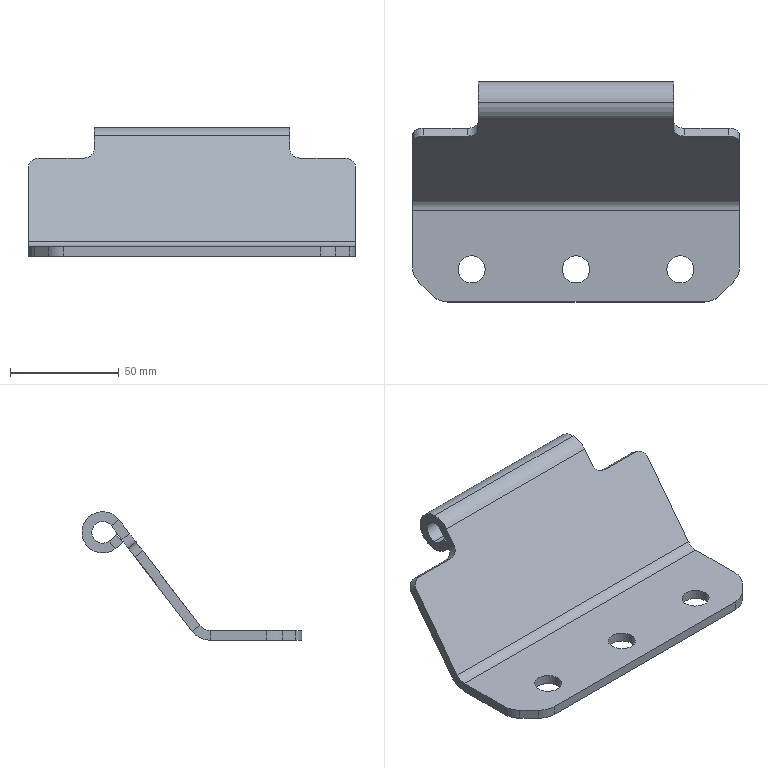Part | SolidWorks | features Fillet 2, ICE 2, Chamfer 1, FlatPattern 1, SMBaseFlange 1, SheetMetal 1 | 1 solid | 46 faces | box 150.4 x 101.2 x 59.2 mm | volume 84882 mm3 | plane 24 | cylinder 22 | commonest cylinder face diameters 10 x7 12.5 x6 20 x4 19 x3 12 x1 21 x1
STEP:
#1=CARTESIAN_POINT('',(41.75,15.,0.));
#2=VERTEX_POINT('',#1);
#3=CARTESIAN_POINT('',(54.25,15.,0.));
#4=VERTEX_POINT('',#3);
#5=CARTESIAN_POINT('',(48.,15.,0.));
#6=DIRECTION('',(0.,0.,1.));
#7=DIRECTION('',(1.,0.,0.));
#8=AXIS2_PLACEMENT_3D('',#5,#6,#7);
#9=CIRCLE('',#8,6.25);
#10=EDGE_CURVE('',#2,#4,#9,.T.);
#11=ORIENTED_EDGE('',*,*,#10,.T.);
#12=CARTESIAN_POINT('',(54.25,15.,-4.5));
#13=VERTEX_POINT('',#12);
#14=CARTESIAN_POINT('',(54.25,15.,54.7));
#15=DIRECTION('',(0.,0.,-1.));
#16=VECTOR('',#15,1000.);
#17=LINE('',#14,#16);
#18=EDGE_CURVE('',#4,#13,#17,.T.);
#19=ORIENTED_EDGE('',*,*,#18,.T.);
#20=CARTESIAN_POINT('',(41.75,15.,-4.5));
#21=VERTEX_POINT('',#20);
#22=CARTESIAN_POINT('',(48.,15.,-4.5));
#23=DIRECTION('',(0.,0.,-1.));
#24=DIRECTION('',(-1.,0.,0.));
#25=AXIS2_PLACEMENT_3D('',#22,#23,#24);
#26=CIRCLE('',#25,6.25);
#27=EDGE_CURVE('',#13,#21,#26,.T.);
#28=ORIENTED_EDGE('',*,*,#27,.T.);
#29=CARTESIAN_POINT('',(41.75,15.,54.7));
#30=DIRECTION('',(0.,0.,-1.));
#31=VECTOR('',#30,1000.);
#32=LINE('',#29,#31);
#33=EDGE_CURVE('',#2,#21,#32,.T.);
#34=ORIENTED_EDGE('',*,*,#33,.F.);
#35=EDGE_LOOP('',(#11,#19,#28,#34));
#36=FACE_OUTER_BOUND('',#35,.T.);
#37=CARTESIAN_POINT('',(48.,15.,54.7));
#38=DIRECTION('',(0.,0.,-1.));
#39=DIRECTION('',(-1.,0.,0.));
#40=AXIS2_PLACEMENT_3D('',#37,#38,#39);
#41=CYLINDRICAL_SURFACE('',#40,6.25);
#42=ADVANCED_FACE('',(#36),#41,.F.);
#43=CARTESIAN_POINT('',(-54.25,15.,0.));
#44=VERTEX_POINT('',#43);
#45=CARTESIAN_POINT('',(-41.75,15.,0.));
#46=VERTEX_POINT('',#45);
#47=CARTESIAN_POINT('',(-48.,15.,0.));
#48=DIRECTION('',(0.,0.,1.));
#49=DIRECTION('',(1.,0.,0.));
#50=AXIS2_PLACEMENT_3D('',#47,#48,#49);
#51=CIRCLE('',#50,6.25);
#52=EDGE_CURVE('',#44,#46,#51,.T.);
#53=ORIENTED_EDGE('',*,*,#52,.T.);
#54=CARTESIAN_POINT('',(-41.75,15.,-4.5));
#55=VERTEX_POINT('',#54);
#56=CARTESIAN_POINT('',(-41.75,15.,54.7));
#57=DIRECTION('',(0.,0.,-1.));
#58=VECTOR('',#57,1000.);
#59=LINE('',#56,#58);
#60=EDGE_CURVE('',#46,#55,#59,.T.);
#61=ORIENTED_EDGE('',*,*,#60,.T.);
#62=CARTESIAN_POINT('',(-54.25,15.,-4.5));
#63=VERTEX_POINT('',#62);
#64=CARTESIAN_POINT('',(-48.,15.,-4.5));
#65=DIRECTION('',(0.,0.,-1.));
#66=DIRECTION('',(-1.,0.,0.));
#67=AXIS2_PLACEMENT_3D('',#64,#65,#66);
#68=CIRCLE('',#67,6.25);
#69=EDGE_CURVE('',#55,#63,#68,.T.);
#70=ORIENTED_EDGE('',*,*,#69,.T.);
#71=CARTESIAN_POINT('',(-54.25,15.,54.7));
#72=DIRECTION('',(0.,0.,-1.));
#73=VECTOR('',#72,1000.);
#74=LINE('',#71,#73);
#75=EDGE_CURVE('',#44,#63,#74,.T.);
#76=ORIENTED_EDGE('',*,*,#75,.F.);
#77=EDGE_LOOP('',(#53,#61,#70,#76));
#78=FACE_OUTER_BOUND('',#77,.T.);
#79=CARTESIAN_POINT('',(-48.,15.,54.7));
#80=DIRECTION('',(0.,0.,-1.));
#81=DIRECTION('',(-1.,0.,0.));
#82=AXIS2_PLACEMENT_3D('',#79,#80,#81);
#83=CYLINDRICAL_SURFACE('',#82,6.25);
#84=ADVANCED_FACE('',(#78),#83,.F.);
#85=CARTESIAN_POINT('',(-6.25,15.,0.));
#86=VERTEX_POINT('',#85);
#87=CARTESIAN_POINT('',(6.25,15.,0.));
#88=VERTEX_POINT('',#87);
#89=CARTESIAN_POINT('',(0.,15.,0.));
#90=DIRECTION('',(0.,0.,1.));
#91=DIRECTION('',(1.,0.,0.));
#92=AXIS2_PLACEMENT_3D('',#89,#90,#91);
#93=CIRCLE('',#92,6.25);
#94=EDGE_CURVE('',#86,#88,#93,.T.);
#95=ORIENTED_EDGE('',*,*,#94,.T.);
#96=CARTESIAN_POINT('',(6.25,15.,-4.5));
#97=VERTEX_POINT('',#96);
#98=CARTESIAN_POINT('',(6.25,15.,54.7));
#99=DIRECTION('',(0.,0.,-1.));
#100=VECTOR('',#99,1000.);
#101=LINE('',#98,#100);
#102=EDGE_CURVE('',#88,#97,#101,.T.);
#103=ORIENTED_EDGE('',*,*,#102,.T.);
#104=CARTESIAN_POINT('',(-6.25,15.,-4.5));
#105=VERTEX_POINT('',#104);
#106=CARTESIAN_POINT('',(0.,15.,-4.5));
#107=DIRECTION('',(0.,0.,-1.));
#108=DIRECTION('',(-1.,0.,0.));
#109=AXIS2_PLACEMENT_3D('',#106,#107,#108);
#110=CIRCLE('',#109,6.25);
#111=EDGE_CURVE('',#97,#105,#110,.T.);
#112=ORIENTED_EDGE('',*,*,#111,.T.);
#113=CARTESIAN_POINT('',(-6.25,15.,54.7));
#114=DIRECTION('',(0.,0.,-1.));
#115=VECTOR('',#114,1000.);
#116=LINE('',#113,#115);
#117=EDGE_CURVE('',#86,#105,#116,.T.);
#118=ORIENTED_EDGE('',*,*,#117,.F.);
#119=EDGE_LOOP('',(#95,#103,#112,#118));
#120=FACE_OUTER_BOUND('',#119,.T.);
#121=CARTESIAN_POINT('',(0.,15.,54.7));
#122=DIRECTION('',(0.,0.,-1.));
#123=DIRECTION('',(-1.,0.,0.));
#124=AXIS2_PLACEMENT_3D('',#121,#122,#123);
#125=CYLINDRICAL_SURFACE('',#124,6.25);
#126=ADVANCED_FACE('',(#120),#125,.F.);
#127=CARTESIAN_POINT('',(45.,88.659,41.231));
#128=VERTEX_POINT('',#127);
#129=CARTESIAN_POINT('',(45.,91.7,40.2));
#130=VERTEX_POINT('',#129);
#131=CARTESIAN_POINT('',(45.,91.7,45.2));
#132=DIRECTION('',(1.,0.,0.));
#133=DIRECTION('',(0.,0.,1.));
#134=AXIS2_PLACEMENT_3D('',#131,#132,#133);
#135=CIRCLE('',#134,5.);
#136=EDGE_CURVE('',#128,#130,#135,.T.);
#137=ORIENTED_EDGE('',*,*,#136,.T.);
#138=CARTESIAN_POINT('',(-45.,91.7,40.2));
#139=VERTEX_POINT('',#138);
#140=CARTESIAN_POINT('',(75.2,91.7,40.2));
#141=DIRECTION('',(-1.,0.,0.));
#142=VECTOR('',#141,1000.);
#143=LINE('',#140,#142);
#144=EDGE_CURVE('',#130,#139,#143,.T.);
#145=ORIENTED_EDGE('',*,*,#144,.T.);
#146=CARTESIAN_POINT('',(-45.,88.659,41.231));
#147=VERTEX_POINT('',#146);
#148=CARTESIAN_POINT('',(-45.,91.7,45.2));
#149=DIRECTION('',(-1.,0.,0.));
#150=DIRECTION('',(0.,0.,-1.));
#151=AXIS2_PLACEMENT_3D('',#148,#149,#150);
#152=CIRCLE('',#151,5.);
#153=EDGE_CURVE('',#139,#147,#152,.T.);
#154=ORIENTED_EDGE('',*,*,#153,.T.);
#155=CARTESIAN_POINT('',(75.2,88.659,41.231));
#156=DIRECTION('',(-1.,0.,0.));
#157=VECTOR('',#156,1000.);
#158=LINE('',#155,#157);
#159=EDGE_CURVE('',#128,#147,#158,.T.);
#160=ORIENTED_EDGE('',*,*,#159,.F.);
#161=EDGE_LOOP('',(#137,#145,#154,#160));
#162=FACE_OUTER_BOUND('',#161,.T.);
#163=CARTESIAN_POINT('',(75.2,91.7,45.2));
#164=DIRECTION('',(-1.,0.,0.));
#165=DIRECTION('',(0.,0.,1.));
#166=AXIS2_PLACEMENT_3D('',#163,#164,#165);
#167=CYLINDRICAL_SURFACE('',#166,5.);
#168=ADVANCED_FACE('',(#162),#167,.F.);
#169=ORIENTED_EDGE('',*,*,#144,.F.);
#170=CARTESIAN_POINT('',(45.,91.7,50.2));
#171=VERTEX_POINT('',#170);
#172=CARTESIAN_POINT('',(45.,91.7,45.2));
#173=DIRECTION('',(1.,0.,0.));
#174=DIRECTION('',(0.,0.,1.));
#175=AXIS2_PLACEMENT_3D('',#172,#173,#174);
#176=CIRCLE('',#175,5.);
#177=EDGE_CURVE('',#130,#171,#176,.T.);
#178=ORIENTED_EDGE('',*,*,#177,.T.);
#179=CARTESIAN_POINT('',(-45.,91.7,50.2));
#180=VERTEX_POINT('',#179);
#181=CARTESIAN_POINT('',(75.2,91.7,50.2));
#182=DIRECTION('',(-1.,0.,0.));
#183=VECTOR('',#182,1000.);
#184=LINE('',#181,#183);
#185=EDGE_CURVE('',#171,#180,#184,.T.);
#186=ORIENTED_EDGE('',*,*,#185,.T.);
#187=CARTESIAN_POINT('',(-45.,91.7,45.2));
#188=DIRECTION('',(-1.,0.,0.));
#189=DIRECTION('',(0.,0.,-1.));
#190=AXIS2_PLACEMENT_3D('',#187,#188,#189);
#191=CIRCLE('',#190,5.);
#192=EDGE_CURVE('',#180,#139,#191,.T.);
#193=ORIENTED_EDGE('',*,*,#192,.T.);
#194=EDGE_LOOP('',(#169,#178,#186,#193));
#195=FACE_OUTER_BOUND('',#194,.T.);
#196=CARTESIAN_POINT('',(75.2,91.7,45.2));
#197=DIRECTION('',(-1.,0.,0.));
#198=DIRECTION('',(0.,0.,1.));
#199=AXIS2_PLACEMENT_3D('',#196,#197,#198);
#200=CYLINDRICAL_SURFACE('',#199,5.);
#201=ADVANCED_FACE('',(#195),#200,.F.);
#202=CARTESIAN_POINT('',(45.,91.7,35.7));
#203=VERTEX_POINT('',#202);
#204=CARTESIAN_POINT('',(45.,91.7,54.7));
#205=VERTEX_POINT('',#204);
#206=CARTESIAN_POINT('',(45.,91.7,45.2));
#207=DIRECTION('',(1.,0.,0.));
#208=DIRECTION('',(0.,0.,1.));
#209=AXIS2_PLACEMENT_3D('',#206,#207,#208);
#210=CIRCLE('',#209,9.5);
#211=EDGE_CURVE('',#203,#205,#210,.T.);
#212=ORIENTED_EDGE('',*,*,#211,.F.);
#213=CARTESIAN_POINT('',(-45.,91.7,35.7));
#214=VERTEX_POINT('',#213);
#215=CARTESIAN_POINT('',(75.2,91.7,35.7));
#216=DIRECTION('',(-1.,0.,0.));
#217=VECTOR('',#216,1000.);
#218=LINE('',#215,#217);
#219=EDGE_CURVE('',#203,#214,#218,.T.);
#220=ORIENTED_EDGE('',*,*,#219,.T.);
#221=CARTESIAN_POINT('',(-45.,91.7,54.7));
#222=VERTEX_POINT('',#221);
#223=CARTESIAN_POINT('',(-45.,91.7,45.2));
#224=DIRECTION('',(-1.,0.,0.));
#225=DIRECTION('',(0.,0.,-1.));
#226=AXIS2_PLACEMENT_3D('',#223,#224,#225);
#227=CIRCLE('',#226,9.5);
#228=EDGE_CURVE('',#222,#214,#227,.T.);
#229=ORIENTED_EDGE('',*,*,#228,.F.);
#230=CARTESIAN_POINT('',(75.2,91.7,54.7));
#231=DIRECTION('',(-1.,0.,0.));
#232=VECTOR('',#231,1000.);
#233=LINE('',#230,#232);
#234=EDGE_CURVE('',#205,#222,#233,.T.);
#235=ORIENTED_EDGE('',*,*,#234,.F.);
#236=EDGE_LOOP('',(#212,#220,#229,#235));
#237=FACE_OUTER_BOUND('',#236,.T.);
#238=CARTESIAN_POINT('',(75.2,91.7,45.2));
#239=DIRECTION('',(-1.,0.,0.));
#240=DIRECTION('',(0.,0.,1.));
#241=AXIS2_PLACEMENT_3D('',#238,#239,#240);
#242=CYLINDRICAL_SURFACE('',#241,9.5);
#243=ADVANCED_FACE('',(#237),#242,.T.);
#244=CARTESIAN_POINT('',(45.,84.159,50.978));
#245=VERTEX_POINT('',#244);
#246=CARTESIAN_POINT('',(45.,91.7,45.2));
#247=DIRECTION('',(1.,0.,0.));
#248=DIRECTION('',(0.,0.,1.));
#249=AXIS2_PLACEMENT_3D('',#246,#247,#248);
#250=CIRCLE('',#249,9.5);
#251=EDGE_CURVE('',#205,#245,#250,.T.);
#252=ORIENTED_EDGE('',*,*,#251,.F.);
#253=ORIENTED_EDGE('',*,*,#234,.T.);
#254=CARTESIAN_POINT('',(-45.,84.159,50.978));
#255=VERTEX_POINT('',#254);
#256=CARTESIAN_POINT('',(-45.,91.7,45.2));
#257=DIRECTION('',(-1.,0.,0.));
#258=DIRECTION('',(0.,0.,-1.));
#259=AXIS2_PLACEMENT_3D('',#256,#257,#258);
#260=CIRCLE('',#259,9.5);
#261=EDGE_CURVE('',#255,#222,#260,.T.);
#262=ORIENTED_EDGE('',*,*,#261,.F.);
#263=CARTESIAN_POINT('',(75.2,84.159,50.978));
#264=DIRECTION('',(-1.,0.,0.));
#265=VECTOR('',#264,1000.);
#266=LINE('',#263,#265);
#267=EDGE_CURVE('',#245,#255,#266,.T.);
#268=ORIENTED_EDGE('',*,*,#267,.F.);
#269=EDGE_LOOP('',(#252,#253,#262,#268));
#270=FACE_OUTER_BOUND('',#269,.T.);
#271=CARTESIAN_POINT('',(75.2,91.7,45.2));
#272=DIRECTION('',(-1.,0.,0.));
#273=DIRECTION('',(0.,0.,1.));
#274=AXIS2_PLACEMENT_3D('',#271,#272,#273);
#275=CYLINDRICAL_SURFACE('',#274,9.5);
#276=ADVANCED_FACE('',(#270),#275,.T.);
#277=CARTESIAN_POINT('',(-45.,85.087,43.968));
#278=VERTEX_POINT('',#277);
#279=CARTESIAN_POINT('',(-45.,88.659,41.231));
#280=DIRECTION('',(0.,-0.7938,0.6082));
#281=VECTOR('',#280,1000.);
#282=LINE('',#279,#281);
#283=EDGE_CURVE('',#147,#278,#282,.T.);
#284=ORIENTED_EDGE('',*,*,#283,.F.);
#285=CARTESIAN_POINT('',(-45.,85.922,37.659));
#286=VERTEX_POINT('',#285);
#287=CARTESIAN_POINT('',(-45.,88.659,41.231));
#288=DIRECTION('',(0.,-0.6082,-0.7938));
#289=VECTOR('',#288,1000.);
#290=LINE('',#287,#289);
#291=EDGE_CURVE('',#147,#286,#290,.T.);
#292=ORIENTED_EDGE('',*,*,#291,.T.);
#293=CARTESIAN_POINT('',(-45.,82.35,40.396));
#294=VERTEX_POINT('',#293);
#295=CARTESIAN_POINT('',(-45.,85.922,37.659));
#296=DIRECTION('',(0.,-0.7938,0.6082));
#297=VECTOR('',#296,1000.);
#298=LINE('',#295,#297);
#299=EDGE_CURVE('',#286,#294,#298,.T.);
#300=ORIENTED_EDGE('',*,*,#299,.T.);
#301=CARTESIAN_POINT('',(-45.,82.35,40.396));
#302=DIRECTION('',(0.,0.6082,0.7938));
#303=VECTOR('',#302,1000.);
#304=LINE('',#301,#303);
#305=EDGE_CURVE('',#294,#278,#304,.T.);
#306=ORIENTED_EDGE('',*,*,#305,.T.);
#307=EDGE_LOOP('',(#284,#292,#300,#306));
#308=FACE_OUTER_BOUND('',#307,.T.);
#309=CARTESIAN_POINT('',(-45.,127.458,29.77));
#310=DIRECTION('',(1.,0.,0.));
#311=DIRECTION('',(0.,0.,-1.));
#312=AXIS2_PLACEMENT_3D('',#309,#310,#311);
#313=PLANE('',#312);
#314=ADVANCED_FACE('',(#308),#313,.F.);
#315=CARTESIAN_POINT('',(-45.,82.865,41.891));
#316=VERTEX_POINT('',#315);
#317=CARTESIAN_POINT('',(-45.,87.731,48.241));
#318=VERTEX_POINT('',#317);
#319=CARTESIAN_POINT('',(-45.,48.672,-2.737));
#320=DIRECTION('',(0.,0.6082,0.7938));
#321=VECTOR('',#320,1000.);
#322=LINE('',#319,#321);
#323=EDGE_CURVE('',#316,#318,#322,.T.);
#324=ORIENTED_EDGE('',*,*,#323,.F.);
#325=CARTESIAN_POINT('',(-45.,79.293,44.628));
#326=VERTEX_POINT('',#325);
#327=CARTESIAN_POINT('',(-45.,79.293,44.628));
#328=DIRECTION('',(0.,-0.7938,0.6082));
#329=VECTOR('',#328,1000.);
#330=LINE('',#327,#329);
#331=EDGE_CURVE('',#316,#326,#330,.T.);
#332=ORIENTED_EDGE('',*,*,#331,.T.);
#333=CARTESIAN_POINT('',(-45.,89.937,58.519));
#334=DIRECTION('',(0.,0.6082,0.7938));
#335=VECTOR('',#334,1000.);
#336=LINE('',#333,#335);
#337=EDGE_CURVE('',#326,#255,#336,.T.);
#338=ORIENTED_EDGE('',*,*,#337,.T.);
#339=CARTESIAN_POINT('',(-45.,84.159,50.978));
#340=DIRECTION('',(0.,0.7938,-0.6082));
#341=VECTOR('',#340,1000.);
#342=LINE('',#339,#341);
#343=EDGE_CURVE('',#255,#318,#342,.T.);
#344=ORIENTED_EDGE('',*,*,#343,.T.);
#345=EDGE_LOOP('',(#324,#332,#338,#344));
#346=FACE_OUTER_BOUND('',#345,.T.);
#347=CARTESIAN_POINT('',(-45.,127.458,29.77));
#348=DIRECTION('',(1.,0.,0.));
#349=DIRECTION('',(0.,0.,-1.));
#350=AXIS2_PLACEMENT_3D('',#347,#348,#349);
#351=PLANE('',#350);
#352=ADVANCED_FACE('',(#346),#351,.F.);
#353=CARTESIAN_POINT('',(45.,82.35,40.396));
#354=VERTEX_POINT('',#353);
#355=CARTESIAN_POINT('',(45.,85.922,37.659));
#356=VERTEX_POINT('',#355);
#357=CARTESIAN_POINT('',(45.,85.922,37.659));
#358=DIRECTION('',(0.,0.7938,-0.6082));
#359=VECTOR('',#358,1000.);
#360=LINE('',#357,#359);
#361=EDGE_CURVE('',#354,#356,#360,.T.);
#362=ORIENTED_EDGE('',*,*,#361,.T.);
#363=CARTESIAN_POINT('',(45.,85.922,37.659));
#364=DIRECTION('',(0.,0.6082,0.7938));
#365=VECTOR('',#364,1000.);
#366=LINE('',#363,#365);
#367=EDGE_CURVE('',#356,#128,#366,.T.);
#368=ORIENTED_EDGE('',*,*,#367,.T.);
#369=CARTESIAN_POINT('',(45.,85.087,43.968));
#370=VERTEX_POINT('',#369);
#371=CARTESIAN_POINT('',(45.,88.659,41.231));
#372=DIRECTION('',(0.,0.7938,-0.6082));
#373=VECTOR('',#372,1000.);
#374=LINE('',#371,#373);
#375=EDGE_CURVE('',#370,#128,#374,.T.);
#376=ORIENTED_EDGE('',*,*,#375,.F.);
#377=CARTESIAN_POINT('',(45.,82.35,40.396));
#378=DIRECTION('',(0.,-0.6082,-0.7938));
#379=VECTOR('',#378,1000.);
#380=LINE('',#377,#379);
#381=EDGE_CURVE('',#370,#354,#380,.T.);
#382=ORIENTED_EDGE('',*,*,#381,.T.);
#383=EDGE_LOOP('',(#362,#368,#376,#382));
#384=FACE_OUTER_BOUND('',#383,.T.);
#385=CARTESIAN_POINT('',(45.,127.458,29.77));
#386=DIRECTION('',(-1.,0.,0.));
#387=DIRECTION('',(0.,0.,1.));
#388=AXIS2_PLACEMENT_3D('',#385,#386,#387);
#389=PLANE('',#388);
#390=ADVANCED_FACE('',(#384),#389,.F.);
#391=CARTESIAN_POINT('',(45.,79.293,44.628));
#392=VERTEX_POINT('',#391);
#393=CARTESIAN_POINT('',(45.,89.937,58.519));
#394=DIRECTION('',(0.,-0.6082,-0.7938));
#395=VECTOR('',#394,1000.);
#396=LINE('',#393,#395);
#397=EDGE_CURVE('',#245,#392,#396,.T.);
#398=ORIENTED_EDGE('',*,*,#397,.T.);
#399=CARTESIAN_POINT('',(45.,82.865,41.891));
#400=VERTEX_POINT('',#399);
#401=CARTESIAN_POINT('',(45.,82.865,41.891));
#402=DIRECTION('',(0.,0.7938,-0.6082));
#403=VECTOR('',#402,1000.);
#404=LINE('',#401,#403);
#405=EDGE_CURVE('',#392,#400,#404,.T.);
#406=ORIENTED_EDGE('',*,*,#405,.T.);
#407=CARTESIAN_POINT('',(45.,87.731,48.241));
#408=VERTEX_POINT('',#407);
#409=CARTESIAN_POINT('',(45.,48.672,-2.737));
#410=DIRECTION('',(0.,-0.6082,-0.7938));
#411=VECTOR('',#410,1000.);
#412=LINE('',#409,#411);
#413=EDGE_CURVE('',#408,#400,#412,.T.);
#414=ORIENTED_EDGE('',*,*,#413,.F.);
#415=CARTESIAN_POINT('',(45.,87.731,48.241));
#416=DIRECTION('',(0.,-0.7938,0.6082));
#417=VECTOR('',#416,1000.);
#418=LINE('',#415,#417);
#419=EDGE_CURVE('',#408,#245,#418,.T.);
#420=ORIENTED_EDGE('',*,*,#419,.T.);
#421=EDGE_LOOP('',(#398,#406,#414,#420));
#422=FACE_OUTER_BOUND('',#421,.T.);
#423=CARTESIAN_POINT('',(45.,127.458,29.77));
#424=DIRECTION('',(-1.,0.,0.));
#425=DIRECTION('',(0.,0.,1.));
#426=AXIS2_PLACEMENT_3D('',#423,#424,#425);
#427=PLANE('',#426);
#428=ADVANCED_FACE('',(#422),#427,.F.);
#429=CARTESIAN_POINT('',(-75.2,46.901,2.351));
#430=VERTEX_POINT('',#429);
#431=CARTESIAN_POINT('',(-75.2,73.211,36.69));
#432=VERTEX_POINT('',#431);
#433=CARTESIAN_POINT('',(-75.2,45.1,0.));
#434=DIRECTION('',(0.,0.6082,0.7938));
#435=VECTOR('',#434,1000.);
#436=LINE('',#433,#435);
#437=EDGE_CURVE('',#430,#432,#436,.T.);
#438=ORIENTED_EDGE('',*,*,#437,.T.);
#439=CARTESIAN_POINT('',(-75.2,76.784,33.953));
#440=VERTEX_POINT('',#439);
#441=CARTESIAN_POINT('',(-75.2,76.784,33.953));
#442=DIRECTION('',(0.,0.7938,-0.6082));
#443=VECTOR('',#442,1000.);
#444=LINE('',#441,#443);
#445=EDGE_CURVE('',#432,#440,#444,.T.);
#446=ORIENTED_EDGE('',*,*,#445,.T.);
#447=CARTESIAN_POINT('',(-75.2,50.473,-0.3861));
#448=VERTEX_POINT('',#447);
#449=CARTESIAN_POINT('',(-75.2,48.672,-2.737));
#450=DIRECTION('',(0.,0.6082,0.7938));
#451=VECTOR('',#450,1000.);
#452=LINE('',#449,#451);
#453=EDGE_CURVE('',#448,#440,#452,.T.);
#454=ORIENTED_EDGE('',*,*,#453,.F.);
#455=CARTESIAN_POINT('',(-75.2,50.473,-0.3861));
#456=DIRECTION('',(0.,-0.7938,0.6082));
#457=VECTOR('',#456,1000.);
#458=LINE('',#455,#457);
#459=EDGE_CURVE('',#448,#430,#458,.T.);
#460=ORIENTED_EDGE('',*,*,#459,.T.);
#461=EDGE_LOOP('',(#438,#446,#454,#460));
#462=FACE_OUTER_BOUND('',#461,.T.);
#463=CARTESIAN_POINT('',(-75.2,88.659,41.231));
#464=DIRECTION('',(-1.,0.,0.));
#465=DIRECTION('',(0.,0.,1.));
#466=AXIS2_PLACEMENT_3D('',#463,#464,#465);
#467=PLANE('',#466);
#468=ADVANCED_FACE('',(#462),#467,.T.);
#469=CARTESIAN_POINT('',(75.2,46.901,2.351));
#470=VERTEX_POINT('',#469);
#471=CARTESIAN_POINT('',(75.2,50.473,-0.3861));
#472=VERTEX_POINT('',#471);
#473=CARTESIAN_POINT('',(75.2,46.901,2.351));
#474=DIRECTION('',(0.,0.7938,-0.6082));
#475=VECTOR('',#474,1000.);
#476=LINE('',#473,#475);
#477=EDGE_CURVE('',#470,#472,#476,.T.);
#478=ORIENTED_EDGE('',*,*,#477,.F.);
#479=CARTESIAN_POINT('',(75.2,42.138,0.));
#480=VERTEX_POINT('',#479);
#481=CARTESIAN_POINT('',(75.2,42.138,6.));
#482=DIRECTION('',(1.,0.,0.));
#483=DIRECTION('',(0.,0.,1.));
#484=AXIS2_PLACEMENT_3D('',#481,#482,#483);
#485=CIRCLE('',#484,6.);
#486=EDGE_CURVE('',#480,#470,#485,.T.);
#487=ORIENTED_EDGE('',*,*,#486,.F.);
#488=CARTESIAN_POINT('',(75.2,42.138,-4.5));
#489=VERTEX_POINT('',#488);
#490=CARTESIAN_POINT('',(75.2,42.138,-4.5));
#491=DIRECTION('',(0.,0.,1.));
#492=VECTOR('',#491,1000.);
#493=LINE('',#490,#492);
#494=EDGE_CURVE('',#489,#480,#493,.T.);
#495=ORIENTED_EDGE('',*,*,#494,.F.);
#496=CARTESIAN_POINT('',(75.2,42.138,6.));
#497=DIRECTION('',(1.,0.,0.));
#498=DIRECTION('',(0.,0.,-1.));
#499=AXIS2_PLACEMENT_3D('',#496,#497,#498);
#500=CIRCLE('',#499,10.5);
#501=EDGE_CURVE('',#489,#472,#500,.T.);
#502=ORIENTED_EDGE('',*,*,#501,.T.);
#503=EDGE_LOOP('',(#478,#487,#495,#502));
#504=FACE_OUTER_BOUND('',#503,.T.);
#505=CARTESIAN_POINT('',(75.2,46.901,2.351));
#506=DIRECTION('',(1.,0.,0.));
#507=DIRECTION('',(0.,0.,-1.));
#508=AXIS2_PLACEMENT_3D('',#505,#506,#507);
#509=PLANE('',#508);
#510=ADVANCED_FACE('',(#504),#509,.T.);
#511=CARTESIAN_POINT('',(75.2,76.784,33.953));
#512=VERTEX_POINT('',#511);
#513=CARTESIAN_POINT('',(75.2,48.672,-2.737));
#514=DIRECTION('',(0.,0.6082,0.7938));
#515=VECTOR('',#514,1000.);
#516=LINE('',#513,#515);
#517=EDGE_CURVE('',#472,#512,#516,.T.);
#518=ORIENTED_EDGE('',*,*,#517,.T.);
#519=CARTESIAN_POINT('',(75.2,73.211,36.69));
#520=VERTEX_POINT('',#519);
#521=CARTESIAN_POINT('',(75.2,73.211,36.69));
#522=DIRECTION('',(0.,-0.7938,0.6082));
#523=VECTOR('',#522,1000.);
#524=LINE('',#521,#523);
#525=EDGE_CURVE('',#512,#520,#524,.T.);
#526=ORIENTED_EDGE('',*,*,#525,.T.);
#527=CARTESIAN_POINT('',(75.2,45.1,0.));
#528=DIRECTION('',(0.,0.6082,0.7938));
#529=VECTOR('',#528,1000.);
#530=LINE('',#527,#529);
#531=EDGE_CURVE('',#470,#520,#530,.T.);
#532=ORIENTED_EDGE('',*,*,#531,.F.);
#533=ORIENTED_EDGE('',*,*,#477,.T.);
#534=EDGE_LOOP('',(#518,#526,#532,#533));
#535=FACE_OUTER_BOUND('',#534,.T.);
#536=CARTESIAN_POINT('',(75.2,42.138,-4.5));
#537=DIRECTION('',(1.,0.,0.));
#538=DIRECTION('',(0.,0.,-1.));
#539=AXIS2_PLACEMENT_3D('',#536,#537,#538);
#540=PLANE('',#539);
#541=ADVANCED_FACE('',(#535),#540,.T.);
#542=CARTESIAN_POINT('',(-75.2,42.138,0.));
#543=VERTEX_POINT('',#542);
#544=CARTESIAN_POINT('',(-75.2,42.138,-4.5));
#545=VERTEX_POINT('',#544);
#546=CARTESIAN_POINT('',(-75.2,42.138,0.));
#547=DIRECTION('',(0.,0.,-1.));
#548=VECTOR('',#547,1000.);
#549=LINE('',#546,#548);
#550=EDGE_CURVE('',#543,#545,#549,.T.);
#551=ORIENTED_EDGE('',*,*,#550,.F.);
#552=CARTESIAN_POINT('',(-75.2,42.138,6.));
#553=DIRECTION('',(1.,0.,0.));
#554=DIRECTION('',(0.,0.,1.));
#555=AXIS2_PLACEMENT_3D('',#552,#553,#554);
#556=CIRCLE('',#555,6.);
#557=EDGE_CURVE('',#543,#430,#556,.T.);
#558=ORIENTED_EDGE('',*,*,#557,.T.);
#559=ORIENTED_EDGE('',*,*,#459,.F.);
#560=CARTESIAN_POINT('',(-75.2,42.138,6.));
#561=DIRECTION('',(1.,0.,0.));
#562=DIRECTION('',(0.,0.,-1.));
#563=AXIS2_PLACEMENT_3D('',#560,#561,#562);
#564=CIRCLE('',#563,10.5);
#565=EDGE_CURVE('',#545,#448,#564,.T.);
#566=ORIENTED_EDGE('',*,*,#565,.F.);
#567=EDGE_LOOP('',(#551,#558,#559,#566));
#568=FACE_OUTER_BOUND('',#567,.T.);
#569=CARTESIAN_POINT('',(-75.2,42.138,0.));
#570=DIRECTION('',(-1.,0.,0.));
#571=DIRECTION('',(0.,0.,1.));
#572=AXIS2_PLACEMENT_3D('',#569,#570,#571);
#573=PLANE('',#572);
#574=ADVANCED_FACE('',(#568),#573,.T.);
#575=CARTESIAN_POINT('',(-75.2,16.142,-4.5));
#576=VERTEX_POINT('',#575);
#577=CARTESIAN_POINT('',(-75.2,0.,-4.5));
#578=DIRECTION('',(0.,1.,0.));
#579=VECTOR('',#578,1000.);
#580=LINE('',#577,#579);
#581=EDGE_CURVE('',#576,#545,#580,.T.);
#582=ORIENTED_EDGE('',*,*,#581,.F.);
#583=CARTESIAN_POINT('',(-75.2,16.142,0.));
#584=VERTEX_POINT('',#583);
#585=CARTESIAN_POINT('',(-75.2,16.142,-0.3861));
#586=DIRECTION('',(0.,0.,1.));
#587=VECTOR('',#586,1000.);
#588=LINE('',#585,#587);
#589=EDGE_CURVE('',#576,#584,#588,.T.);
#590=ORIENTED_EDGE('',*,*,#589,.T.);
#591=CARTESIAN_POINT('',(-75.2,0.,0.));
#592=DIRECTION('',(0.,1.,0.));
#593=VECTOR('',#592,1000.);
#594=LINE('',#591,#593);
#595=EDGE_CURVE('',#584,#543,#594,.T.);
#596=ORIENTED_EDGE('',*,*,#595,.T.);
#597=ORIENTED_EDGE('',*,*,#550,.T.);
#598=EDGE_LOOP('',(#582,#590,#596,#597));
#599=FACE_OUTER_BOUND('',#598,.T.);
#600=CARTESIAN_POINT('',(-75.2,50.473,-0.3861));
#601=DIRECTION('',(-1.,0.,0.));
#602=DIRECTION('',(0.,0.,1.));
#603=AXIS2_PLACEMENT_3D('',#600,#601,#602);
#604=PLANE('',#603);
#605=ADVANCED_FACE('',(#599),#604,.T.);
#606=ORIENTED_EDGE('',*,*,#159,.T.);
#607=ORIENTED_EDGE('',*,*,#283,.T.);
#608=CARTESIAN_POINT('',(75.2,85.087,43.968));
#609=DIRECTION('',(-1.,0.,0.));
#610=VECTOR('',#609,1000.);
#611=LINE('',#608,#610);
#612=EDGE_CURVE('',#370,#278,#611,.T.);
#613=ORIENTED_EDGE('',*,*,#612,.F.);
#614=ORIENTED_EDGE('',*,*,#375,.T.);
#615=EDGE_LOOP('',(#606,#607,#613,#614));
#616=FACE_OUTER_BOUND('',#615,.T.);
#617=CARTESIAN_POINT('',(75.2,88.659,41.231));
#618=DIRECTION('',(0.,-0.6082,-0.7938));
#619=DIRECTION('',(0.,0.7938,-0.6082));
#620=AXIS2_PLACEMENT_3D('',#617,#618,#619);
#621=PLANE('',#620);
#622=ADVANCED_FACE('',(#616),#621,.F.);
#623=ORIENTED_EDGE('',*,*,#305,.F.);
#624=CARTESIAN_POINT('',(75.2,82.35,40.396));
#625=DIRECTION('',(-1.,0.,0.));
#626=VECTOR('',#625,1000.);
#627=LINE('',#624,#626);
#628=EDGE_CURVE('',#354,#294,#627,.T.);
#629=ORIENTED_EDGE('',*,*,#628,.F.);
#630=ORIENTED_EDGE('',*,*,#381,.F.);
#631=ORIENTED_EDGE('',*,*,#612,.T.);
#632=EDGE_LOOP('',(#623,#629,#630,#631));
#633=FACE_OUTER_BOUND('',#632,.T.);
#634=CARTESIAN_POINT('',(75.2,82.35,40.396));
#635=DIRECTION('',(0.,-0.7938,0.6082));
#636=DIRECTION('',(0.,-0.6082,-0.7938));
#637=AXIS2_PLACEMENT_3D('',#634,#635,#636);
#638=PLANE('',#637);
#639=ADVANCED_FACE('',(#633),#638,.T.);
#640=ORIENTED_EDGE('',*,*,#299,.F.);
#641=CARTESIAN_POINT('',(75.2,85.922,37.659));
#642=DIRECTION('',(-1.,0.,0.));
#643=VECTOR('',#642,1000.);
#644=LINE('',#641,#643);
#645=EDGE_CURVE('',#356,#286,#644,.T.);
#646=ORIENTED_EDGE('',*,*,#645,.F.);
#647=ORIENTED_EDGE('',*,*,#361,.F.);
#648=ORIENTED_EDGE('',*,*,#628,.T.);
#649=EDGE_LOOP('',(#640,#646,#647,#648));
#650=FACE_OUTER_BOUND('',#649,.T.);
#651=CARTESIAN_POINT('',(75.2,85.922,37.659));
#652=DIRECTION('',(0.,-0.6082,-0.7938));
#653=DIRECTION('',(0.,0.7938,-0.6082));
#654=AXIS2_PLACEMENT_3D('',#651,#652,#653);
#655=PLANE('',#654);
#656=ADVANCED_FACE('',(#650),#655,.T.);
#657=ORIENTED_EDGE('',*,*,#219,.F.);
#658=CARTESIAN_POINT('',(45.,91.7,45.2));
#659=DIRECTION('',(1.,0.,0.));
#660=DIRECTION('',(0.,0.,1.));
#661=AXIS2_PLACEMENT_3D('',#658,#659,#660);
#662=CIRCLE('',#661,9.5);
#663=EDGE_CURVE('',#356,#203,#662,.T.);
#664=ORIENTED_EDGE('',*,*,#663,.F.);
#665=ORIENTED_EDGE('',*,*,#645,.T.);
#666=CARTESIAN_POINT('',(-45.,91.7,45.2));
#667=DIRECTION('',(-1.,0.,0.));
#668=DIRECTION('',(0.,0.,-1.));
#669=AXIS2_PLACEMENT_3D('',#666,#667,#668);
#670=CIRCLE('',#669,9.5);
#671=EDGE_CURVE('',#214,#286,#670,.T.);
#672=ORIENTED_EDGE('',*,*,#671,.F.);
#673=EDGE_LOOP('',(#657,#664,#665,#672));
#674=FACE_OUTER_BOUND('',#673,.T.);
#675=CARTESIAN_POINT('',(75.2,91.7,45.2));
#676=DIRECTION('',(-1.,0.,0.));
#677=DIRECTION('',(0.,0.,1.));
#678=AXIS2_PLACEMENT_3D('',#675,#676,#677);
#679=CYLINDRICAL_SURFACE('',#678,9.5);
#680=ADVANCED_FACE('',(#674),#679,.T.);
#681=ORIENTED_EDGE('',*,*,#531,.T.);
#682=CARTESIAN_POINT('',(70.2,76.252,40.659));
#683=VERTEX_POINT('',#682);
#684=CARTESIAN_POINT('',(70.2,73.211,36.69));
#685=DIRECTION('',(0.,-0.7938,0.6082));
#686=DIRECTION('',(0.,-0.6082,-0.7938));
#687=AXIS2_PLACEMENT_3D('',#684,#685,#686);
#688=CIRCLE('',#687,5.);
#689=EDGE_CURVE('',#520,#683,#688,.T.);
#690=ORIENTED_EDGE('',*,*,#689,.T.);
#691=CARTESIAN_POINT('',(50.,76.252,40.659));
#692=VERTEX_POINT('',#691);
#693=CARTESIAN_POINT('',(75.2,76.252,40.659));
#694=DIRECTION('',(1.,0.,0.));
#695=VECTOR('',#694,1000.);
#696=LINE('',#693,#695);
#697=EDGE_CURVE('',#692,#683,#696,.T.);
#698=ORIENTED_EDGE('',*,*,#697,.F.);
#699=CARTESIAN_POINT('',(50.,79.293,44.628));
#700=DIRECTION('',(0.,0.7938,-0.6082));
#701=DIRECTION('',(0.,-0.6082,-0.7938));
#702=AXIS2_PLACEMENT_3D('',#699,#700,#701);
#703=CIRCLE('',#702,5.);
#704=EDGE_CURVE('',#692,#392,#703,.T.);
#705=ORIENTED_EDGE('',*,*,#704,.T.);
#706=ORIENTED_EDGE('',*,*,#397,.F.);
#707=ORIENTED_EDGE('',*,*,#267,.T.);
#708=ORIENTED_EDGE('',*,*,#337,.F.);
#709=CARTESIAN_POINT('',(-50.,76.252,40.659));
#710=VERTEX_POINT('',#709);
#711=CARTESIAN_POINT('',(-50.,79.293,44.628));
#712=DIRECTION('',(0.,0.7938,-0.6082));
#713=DIRECTION('',(0.,-0.6082,-0.7938));
#714=AXIS2_PLACEMENT_3D('',#711,#712,#713);
#715=CIRCLE('',#714,5.);
#716=EDGE_CURVE('',#326,#710,#715,.T.);
#717=ORIENTED_EDGE('',*,*,#716,.T.);
#718=CARTESIAN_POINT('',(-70.2,76.252,40.659));
#719=VERTEX_POINT('',#718);
#720=CARTESIAN_POINT('',(-75.2,76.252,40.659));
#721=DIRECTION('',(1.,0.,0.));
#722=VECTOR('',#721,1000.);
#723=LINE('',#720,#722);
#724=EDGE_CURVE('',#719,#710,#723,.T.);
#725=ORIENTED_EDGE('',*,*,#724,.F.);
#726=CARTESIAN_POINT('',(-70.2,73.211,36.69));
#727=DIRECTION('',(0.,-0.7938,0.6082));
#728=DIRECTION('',(0.,-0.6082,-0.7938));
#729=AXIS2_PLACEMENT_3D('',#726,#727,#728);
#730=CIRCLE('',#729,5.);
#731=EDGE_CURVE('',#719,#432,#730,.T.);
#732=ORIENTED_EDGE('',*,*,#731,.T.);
#733=ORIENTED_EDGE('',*,*,#437,.F.);
#734=CARTESIAN_POINT('',(75.2,46.901,2.351));
#735=DIRECTION('',(-1.,0.,0.));
#736=VECTOR('',#735,1000.);
#737=LINE('',#734,#736);
#738=EDGE_CURVE('',#470,#430,#737,.T.);
#739=ORIENTED_EDGE('',*,*,#738,.F.);
#740=EDGE_LOOP('',(#681,#690,#698,#705,#706,#707,#708,#717,#725,#732,#733,#739));
#741=FACE_OUTER_BOUND('',#740,.T.);
#742=CARTESIAN_POINT('',(75.2,45.1,0.));
#743=DIRECTION('',(0.,-0.7938,0.6082));
#744=DIRECTION('',(0.,-0.6082,-0.7938));
#745=AXIS2_PLACEMENT_3D('',#742,#743,#744);
#746=PLANE('',#745);
#747=ADVANCED_FACE('',(#741),#746,.T.);
#748=ORIENTED_EDGE('',*,*,#557,.F.);
#749=CARTESIAN_POINT('',(75.2,42.138,0.));
#750=DIRECTION('',(-1.,0.,0.));
#751=VECTOR('',#750,1000.);
#752=LINE('',#749,#751);
#753=EDGE_CURVE('',#480,#543,#752,.T.);
#754=ORIENTED_EDGE('',*,*,#753,.F.);
#755=ORIENTED_EDGE('',*,*,#486,.T.);
#756=ORIENTED_EDGE('',*,*,#738,.T.);
#757=EDGE_LOOP('',(#748,#754,#755,#756));
#758=FACE_OUTER_BOUND('',#757,.T.);
#759=CARTESIAN_POINT('',(75.2,42.138,6.));
#760=DIRECTION('',(-1.,0.,0.));
#761=DIRECTION('',(0.,0.,1.));
#762=AXIS2_PLACEMENT_3D('',#759,#760,#761);
#763=CYLINDRICAL_SURFACE('',#762,6.);
#764=ADVANCED_FACE('',(#758),#763,.F.);
#765=ORIENTED_EDGE('',*,*,#10,.F.);
#766=CARTESIAN_POINT('',(48.,15.,0.));
#767=DIRECTION('',(0.,0.,1.));
#768=DIRECTION('',(1.,0.,0.));
#769=AXIS2_PLACEMENT_3D('',#766,#767,#768);
#770=CIRCLE('',#769,6.25);
#771=EDGE_CURVE('',#4,#2,#770,.T.);
#772=ORIENTED_EDGE('',*,*,#771,.F.);
#773=EDGE_LOOP('',(#765,#772));
#774=FACE_BOUND('',#773,.T.);
#775=ORIENTED_EDGE('',*,*,#52,.F.);
#776=CARTESIAN_POINT('',(-48.,15.,0.));
#777=DIRECTION('',(0.,0.,1.));
#778=DIRECTION('',(1.,0.,0.));
#779=AXIS2_PLACEMENT_3D('',#776,#777,#778);
#780=CIRCLE('',#779,6.25);
#781=EDGE_CURVE('',#46,#44,#780,.T.);
#782=ORIENTED_EDGE('',*,*,#781,.F.);
#783=EDGE_LOOP('',(#775,#782));
#784=FACE_BOUND('',#783,.T.);
#785=ORIENTED_EDGE('',*,*,#94,.F.);
#786=CARTESIAN_POINT('',(0.,15.,0.));
#787=DIRECTION('',(0.,0.,1.));
#788=DIRECTION('',(1.,0.,0.));
#789=AXIS2_PLACEMENT_3D('',#786,#787,#788);
#790=CIRCLE('',#789,6.25);
#791=EDGE_CURVE('',#88,#86,#790,.T.);
#792=ORIENTED_EDGE('',*,*,#791,.F.);
#793=EDGE_LOOP('',(#785,#792));
#794=FACE_BOUND('',#793,.T.);
#795=CARTESIAN_POINT('',(59.058,0.,0.));
#796=VERTEX_POINT('',#795);
#797=CARTESIAN_POINT('',(-59.058,0.,0.));
#798=VERTEX_POINT('',#797);
#799=CARTESIAN_POINT('',(75.2,0.,0.));
#800=DIRECTION('',(-1.,0.,0.));
#801=VECTOR('',#800,1000.);
#802=LINE('',#799,#801);
#803=EDGE_CURVE('',#796,#798,#802,.T.);
#804=ORIENTED_EDGE('',*,*,#803,.F.);
#805=CARTESIAN_POINT('',(66.129,2.929,0.));
#806=VERTEX_POINT('',#805);
#807=CARTESIAN_POINT('',(59.058,10.,0.));
#808=DIRECTION('',(0.,0.,1.));
#809=DIRECTION('',(1.,0.,0.));
#810=AXIS2_PLACEMENT_3D('',#807,#808,#809);
#811=CIRCLE('',#810,10.);
#812=EDGE_CURVE('',#796,#806,#811,.T.);
#813=ORIENTED_EDGE('',*,*,#812,.T.);
#814=CARTESIAN_POINT('',(72.271,9.071,0.));
#815=VERTEX_POINT('',#814);
#816=CARTESIAN_POINT('',(69.2,6.,0.));
#817=DIRECTION('',(0.7071,0.7071,0.));
#818=VECTOR('',#817,1000.);
#819=LINE('',#816,#818);
#820=EDGE_CURVE('',#806,#815,#819,.T.);
#821=ORIENTED_EDGE('',*,*,#820,.T.);
#822=CARTESIAN_POINT('',(75.2,16.142,0.));
#823=VERTEX_POINT('',#822);
#824=CARTESIAN_POINT('',(65.2,16.142,0.));
#825=DIRECTION('',(0.,0.,1.));
#826=DIRECTION('',(1.,0.,0.));
#827=AXIS2_PLACEMENT_3D('',#824,#825,#826);
#828=CIRCLE('',#827,10.);
#829=EDGE_CURVE('',#815,#823,#828,.T.);
#830=ORIENTED_EDGE('',*,*,#829,.T.);
#831=CARTESIAN_POINT('',(75.2,0.,0.));
#832=DIRECTION('',(0.,1.,0.));
#833=VECTOR('',#832,1000.);
#834=LINE('',#831,#833);
#835=EDGE_CURVE('',#823,#480,#834,.T.);
#836=ORIENTED_EDGE('',*,*,#835,.T.);
#837=ORIENTED_EDGE('',*,*,#753,.T.);
#838=ORIENTED_EDGE('',*,*,#595,.F.);
#839=CARTESIAN_POINT('',(-72.271,9.071,0.));
#840=VERTEX_POINT('',#839);
#841=CARTESIAN_POINT('',(-65.2,16.142,0.));
#842=DIRECTION('',(0.,0.,1.));
#843=DIRECTION('',(1.,0.,0.));
#844=AXIS2_PLACEMENT_3D('',#841,#842,#843);
#845=CIRCLE('',#844,10.);
#846=EDGE_CURVE('',#584,#840,#845,.T.);
#847=ORIENTED_EDGE('',*,*,#846,.T.);
#848=CARTESIAN_POINT('',(-66.129,2.929,0.));
#849=VERTEX_POINT('',#848);
#850=CARTESIAN_POINT('',(6.,-69.2,0.));
#851=DIRECTION('',(0.7071,-0.7071,0.));
#852=VECTOR('',#851,1000.);
#853=LINE('',#850,#852);
#854=EDGE_CURVE('',#840,#849,#853,.T.);
#855=ORIENTED_EDGE('',*,*,#854,.T.);
#856=CARTESIAN_POINT('',(-59.058,10.,0.));
#857=DIRECTION('',(0.,0.,1.));
#858=DIRECTION('',(1.,0.,0.));
#859=AXIS2_PLACEMENT_3D('',#856,#857,#858);
#860=CIRCLE('',#859,10.);
#861=EDGE_CURVE('',#849,#798,#860,.T.);
#862=ORIENTED_EDGE('',*,*,#861,.T.);
#863=EDGE_LOOP('',(#804,#813,#821,#830,#836,#837,#838,#847,#855,#862));
#864=FACE_OUTER_BOUND('',#863,.T.);
#865=CARTESIAN_POINT('',(75.2,0.,0.));
#866=DIRECTION('',(0.,0.,1.));
#867=DIRECTION('',(1.,0.,0.));
#868=AXIS2_PLACEMENT_3D('',#865,#866,#867);
#869=PLANE('',#868);
#870=ADVANCED_FACE('',(#774,#784,#794,#864),#869,.T.);
#871=CARTESIAN_POINT('',(59.058,0.,-4.5));
#872=VERTEX_POINT('',#871);
#873=CARTESIAN_POINT('',(-59.058,0.,-4.5));
#874=VERTEX_POINT('',#873);
#875=CARTESIAN_POINT('',(75.2,0.,-4.5));
#876=DIRECTION('',(-1.,0.,0.));
#877=VECTOR('',#876,1000.);
#878=LINE('',#875,#877);
#879=EDGE_CURVE('',#872,#874,#878,.T.);
#880=ORIENTED_EDGE('',*,*,#879,.F.);
#881=CARTESIAN_POINT('',(59.058,0.,-4.5));
#882=DIRECTION('',(0.,0.,1.));
#883=VECTOR('',#882,1000.);
#884=LINE('',#881,#883);
#885=EDGE_CURVE('',#872,#796,#884,.T.);
#886=ORIENTED_EDGE('',*,*,#885,.T.);
#887=ORIENTED_EDGE('',*,*,#803,.T.);
#888=CARTESIAN_POINT('',(-59.058,0.,-4.5));
#889=DIRECTION('',(0.,0.,-1.));
#890=VECTOR('',#889,1000.);
#891=LINE('',#888,#890);
#892=EDGE_CURVE('',#798,#874,#891,.T.);
#893=ORIENTED_EDGE('',*,*,#892,.T.);
#894=EDGE_LOOP('',(#880,#886,#887,#893));
#895=FACE_OUTER_BOUND('',#894,.T.);
#896=CARTESIAN_POINT('',(75.2,0.,-4.5));
#897=DIRECTION('',(0.,-1.,0.));
#898=DIRECTION('',(0.,0.,-1.));
#899=AXIS2_PLACEMENT_3D('',#896,#897,#898);
#900=PLANE('',#899);
#901=ADVANCED_FACE('',(#895),#900,.T.);
#902=CARTESIAN_POINT('',(48.,15.,-4.5));
#903=DIRECTION('',(0.,0.,-1.));
#904=DIRECTION('',(-1.,0.,0.));
#905=AXIS2_PLACEMENT_3D('',#902,#903,#904);
#906=CIRCLE('',#905,6.25);
#907=EDGE_CURVE('',#21,#13,#906,.T.);
#908=ORIENTED_EDGE('',*,*,#907,.F.);
#909=ORIENTED_EDGE('',*,*,#27,.F.);
#910=EDGE_LOOP('',(#908,#909));
#911=FACE_BOUND('',#910,.T.);
#912=CARTESIAN_POINT('',(-48.,15.,-4.5));
#913=DIRECTION('',(0.,0.,-1.));
#914=DIRECTION('',(-1.,0.,0.));
#915=AXIS2_PLACEMENT_3D('',#912,#913,#914);
#916=CIRCLE('',#915,6.25);
#917=EDGE_CURVE('',#63,#55,#916,.T.);
#918=ORIENTED_EDGE('',*,*,#917,.F.);
#919=ORIENTED_EDGE('',*,*,#69,.F.);
#920=EDGE_LOOP('',(#918,#919));
#921=FACE_BOUND('',#920,.T.);
#922=CARTESIAN_POINT('',(0.,15.,-4.5));
#923=DIRECTION('',(0.,0.,-1.));
#924=DIRECTION('',(-1.,0.,0.));
#925=AXIS2_PLACEMENT_3D('',#922,#923,#924);
#926=CIRCLE('',#925,6.25);
#927=EDGE_CURVE('',#105,#97,#926,.T.);
#928=ORIENTED_EDGE('',*,*,#927,.F.);
#929=ORIENTED_EDGE('',*,*,#111,.F.);
#930=EDGE_LOOP('',(#928,#929));
#931=FACE_BOUND('',#930,.T.);
#932=CARTESIAN_POINT('',(72.271,9.071,-4.5));
#933=VERTEX_POINT('',#932);
#934=CARTESIAN_POINT('',(66.129,2.929,-4.5));
#935=VERTEX_POINT('',#934);
#936=CARTESIAN_POINT('',(63.2,0.,-4.5));
#937=DIRECTION('',(-0.7071,-0.7071,0.));
#938=VECTOR('',#937,1000.);
#939=LINE('',#936,#938);
#940=EDGE_CURVE('',#933,#935,#939,.T.);
#941=ORIENTED_EDGE('',*,*,#940,.T.);
#942=CARTESIAN_POINT('',(59.058,10.,-4.5));
#943=DIRECTION('',(0.,0.,-1.));
#944=DIRECTION('',(1.,0.,0.));
#945=AXIS2_PLACEMENT_3D('',#942,#943,#944);
#946=CIRCLE('',#945,10.);
#947=EDGE_CURVE('',#935,#872,#946,.T.);
#948=ORIENTED_EDGE('',*,*,#947,.T.);
#949=ORIENTED_EDGE('',*,*,#879,.T.);
#950=CARTESIAN_POINT('',(-66.129,2.929,-4.5));
#951=VERTEX_POINT('',#950);
#952=CARTESIAN_POINT('',(-59.058,10.,-4.5));
#953=DIRECTION('',(0.,0.,-1.));
#954=DIRECTION('',(1.,0.,0.));
#955=AXIS2_PLACEMENT_3D('',#952,#953,#954);
#956=CIRCLE('',#955,10.);
#957=EDGE_CURVE('',#874,#951,#956,.T.);
#958=ORIENTED_EDGE('',*,*,#957,.T.);
#959=CARTESIAN_POINT('',(-72.271,9.071,-4.5));
#960=VERTEX_POINT('',#959);
#961=CARTESIAN_POINT('',(-75.2,12.,-4.5));
#962=DIRECTION('',(-0.7071,0.7071,0.));
#963=VECTOR('',#962,1000.);
#964=LINE('',#961,#963);
#965=EDGE_CURVE('',#951,#960,#964,.T.);
#966=ORIENTED_EDGE('',*,*,#965,.T.);
#967=CARTESIAN_POINT('',(-65.2,16.142,-4.5));
#968=DIRECTION('',(0.,0.,-1.));
#969=DIRECTION('',(1.,0.,0.));
#970=AXIS2_PLACEMENT_3D('',#967,#968,#969);
#971=CIRCLE('',#970,10.);
#972=EDGE_CURVE('',#960,#576,#971,.T.);
#973=ORIENTED_EDGE('',*,*,#972,.T.);
#974=ORIENTED_EDGE('',*,*,#581,.T.);
#975=CARTESIAN_POINT('',(75.2,42.138,-4.5));
#976=DIRECTION('',(-1.,0.,0.));
#977=VECTOR('',#976,1000.);
#978=LINE('',#975,#977);
#979=EDGE_CURVE('',#489,#545,#978,.T.);
#980=ORIENTED_EDGE('',*,*,#979,.F.);
#981=CARTESIAN_POINT('',(75.2,16.142,-4.5));
#982=VERTEX_POINT('',#981);
#983=CARTESIAN_POINT('',(75.2,0.,-4.5));
#984=DIRECTION('',(0.,1.,0.));
#985=VECTOR('',#984,1000.);
#986=LINE('',#983,#985);
#987=EDGE_CURVE('',#982,#489,#986,.T.);
#988=ORIENTED_EDGE('',*,*,#987,.F.);
#989=CARTESIAN_POINT('',(65.2,16.142,-4.5));
#990=DIRECTION('',(0.,0.,-1.));
#991=DIRECTION('',(1.,0.,0.));
#992=AXIS2_PLACEMENT_3D('',#989,#990,#991);
#993=CIRCLE('',#992,10.);
#994=EDGE_CURVE('',#982,#933,#993,.T.);
#995=ORIENTED_EDGE('',*,*,#994,.T.);
#996=EDGE_LOOP('',(#941,#948,#949,#958,#966,#973,#974,#980,#988,#995));
#997=FACE_OUTER_BOUND('',#996,.T.);
#998=CARTESIAN_POINT('',(75.2,0.,-4.5));
#999=DIRECTION('',(0.,0.,1.));
#1000=DIRECTION('',(1.,0.,0.));
#1001=AXIS2_PLACEMENT_3D('',#998,#999,#1000);
#1002=PLANE('',#1001);
#1003=ADVANCED_FACE('',(#911,#921,#931,#997),#1002,.F.);
#1004=ORIENTED_EDGE('',*,*,#565,.T.);
#1005=CARTESIAN_POINT('',(75.2,50.473,-0.3861));
#1006=DIRECTION('',(-1.,0.,0.));
#1007=VECTOR('',#1006,1000.);
#1008=LINE('',#1005,#1007);
#1009=EDGE_CURVE('',#472,#448,#1008,.T.);
#1010=ORIENTED_EDGE('',*,*,#1009,.F.);
#1011=ORIENTED_EDGE('',*,*,#501,.F.);
#1012=ORIENTED_EDGE('',*,*,#979,.T.);
#1013=EDGE_LOOP('',(#1004,#1010,#1011,#1012));
#1014=FACE_OUTER_BOUND('',#1013,.T.);
#1015=CARTESIAN_POINT('',(75.2,42.138,6.));
#1016=DIRECTION('',(-1.,0.,0.));
#1017=DIRECTION('',(0.,0.,1.));
#1018=AXIS2_PLACEMENT_3D('',#1015,#1016,#1017);
#1019=CYLINDRICAL_SURFACE('',#1018,10.5);
#1020=ADVANCED_FACE('',(#1014),#1019,.T.);
#1021=CARTESIAN_POINT('',(50.,79.825,37.922));
#1022=VERTEX_POINT('',#1021);
#1023=CARTESIAN_POINT('',(70.2,79.825,37.922));
#1024=VERTEX_POINT('',#1023);
#1025=CARTESIAN_POINT('',(75.2,79.825,37.922));
#1026=DIRECTION('',(1.,0.,0.));
#1027=VECTOR('',#1026,1000.);
#1028=LINE('',#1025,#1027);
#1029=EDGE_CURVE('',#1022,#1024,#1028,.T.);
#1030=ORIENTED_EDGE('',*,*,#1029,.T.);
#1031=CARTESIAN_POINT('',(70.2,76.784,33.953));
#1032=DIRECTION('',(0.,0.7938,-0.6082));
#1033=DIRECTION('',(0.,-0.6082,-0.7938));
#1034=AXIS2_PLACEMENT_3D('',#1031,#1032,#1033);
#1035=CIRCLE('',#1034,5.);
#1036=EDGE_CURVE('',#1024,#512,#1035,.T.);
#1037=ORIENTED_EDGE('',*,*,#1036,.T.);
#1038=ORIENTED_EDGE('',*,*,#517,.F.);
#1039=ORIENTED_EDGE('',*,*,#1009,.T.);
#1040=ORIENTED_EDGE('',*,*,#453,.T.);
#1041=CARTESIAN_POINT('',(-70.2,79.825,37.922));
#1042=VERTEX_POINT('',#1041);
#1043=CARTESIAN_POINT('',(-70.2,76.784,33.953));
#1044=DIRECTION('',(0.,0.7938,-0.6082));
#1045=DIRECTION('',(0.,-0.6082,-0.7938));
#1046=AXIS2_PLACEMENT_3D('',#1043,#1044,#1045);
#1047=CIRCLE('',#1046,5.);
#1048=EDGE_CURVE('',#440,#1042,#1047,.T.);
#1049=ORIENTED_EDGE('',*,*,#1048,.T.);
#1050=CARTESIAN_POINT('',(-50.,79.825,37.922));
#1051=VERTEX_POINT('',#1050);
#1052=CARTESIAN_POINT('',(75.2,79.825,37.922));
#1053=DIRECTION('',(1.,0.,0.));
#1054=VECTOR('',#1053,1000.);
#1055=LINE('',#1052,#1054);
#1056=EDGE_CURVE('',#1042,#1051,#1055,.T.);
#1057=ORIENTED_EDGE('',*,*,#1056,.T.);
#1058=CARTESIAN_POINT('',(-50.,82.865,41.891));
#1059=DIRECTION('',(0.,-0.7938,0.6082));
#1060=DIRECTION('',(0.,-0.6082,-0.7938));
#1061=AXIS2_PLACEMENT_3D('',#1058,#1059,#1060);
#1062=CIRCLE('',#1061,5.);
#1063=EDGE_CURVE('',#1051,#316,#1062,.T.);
#1064=ORIENTED_EDGE('',*,*,#1063,.T.);
#1065=ORIENTED_EDGE('',*,*,#323,.T.);
#1066=CARTESIAN_POINT('',(75.2,87.731,48.241));
#1067=DIRECTION('',(-1.,0.,0.));
#1068=VECTOR('',#1067,1000.);
#1069=LINE('',#1066,#1068);
#1070=EDGE_CURVE('',#408,#318,#1069,.T.);
#1071=ORIENTED_EDGE('',*,*,#1070,.F.);
#1072=ORIENTED_EDGE('',*,*,#413,.T.);
#1073=CARTESIAN_POINT('',(50.,82.865,41.891));
#1074=DIRECTION('',(0.,-0.7938,0.6082));
#1075=DIRECTION('',(0.,-0.6082,-0.7938));
#1076=AXIS2_PLACEMENT_3D('',#1073,#1074,#1075);
#1077=CIRCLE('',#1076,5.);
#1078=EDGE_CURVE('',#400,#1022,#1077,.T.);
#1079=ORIENTED_EDGE('',*,*,#1078,.T.);
#1080=EDGE_LOOP('',(#1030,#1037,#1038,#1039,#1040,#1049,#1057,#1064,#1065,#1071,#1072,#1079));
#1081=FACE_OUTER_BOUND('',#1080,.T.);
#1082=CARTESIAN_POINT('',(75.2,48.672,-2.737));
#1083=DIRECTION('',(0.,-0.7938,0.6082));
#1084=DIRECTION('',(0.,-0.6082,-0.7938));
#1085=AXIS2_PLACEMENT_3D('',#1082,#1083,#1084);
#1086=PLANE('',#1085);
#1087=ADVANCED_FACE('',(#1081),#1086,.F.);
#1088=ORIENTED_EDGE('',*,*,#185,.F.);
#1089=CARTESIAN_POINT('',(45.,91.7,45.2));
#1090=DIRECTION('',(1.,0.,0.));
#1091=DIRECTION('',(0.,0.,1.));
#1092=AXIS2_PLACEMENT_3D('',#1089,#1090,#1091);
#1093=CIRCLE('',#1092,5.);
#1094=EDGE_CURVE('',#171,#408,#1093,.T.);
#1095=ORIENTED_EDGE('',*,*,#1094,.T.);
#1096=ORIENTED_EDGE('',*,*,#1070,.T.);
#1097=CARTESIAN_POINT('',(-45.,91.7,45.2));
#1098=DIRECTION('',(-1.,0.,0.));
#1099=DIRECTION('',(0.,0.,-1.));
#1100=AXIS2_PLACEMENT_3D('',#1097,#1098,#1099);
#1101=CIRCLE('',#1100,5.);
#1102=EDGE_CURVE('',#318,#180,#1101,.T.);
#1103=ORIENTED_EDGE('',*,*,#1102,.T.);
#1104=EDGE_LOOP('',(#1088,#1095,#1096,#1103));
#1105=FACE_OUTER_BOUND('',#1104,.T.);
#1106=CARTESIAN_POINT('',(75.2,91.7,45.2));
#1107=DIRECTION('',(-1.,0.,0.));
#1108=DIRECTION('',(0.,0.,1.));
#1109=AXIS2_PLACEMENT_3D('',#1106,#1107,#1108);
#1110=CYLINDRICAL_SURFACE('',#1109,5.);
#1111=ADVANCED_FACE('',(#1105),#1110,.F.);
#1112=ORIENTED_EDGE('',*,*,#835,.F.);
#1113=CARTESIAN_POINT('',(75.2,16.142,-4.5));
#1114=DIRECTION('',(0.,0.,-1.));
#1115=VECTOR('',#1114,1000.);
#1116=LINE('',#1113,#1115);
#1117=EDGE_CURVE('',#823,#982,#1116,.T.);
#1118=ORIENTED_EDGE('',*,*,#1117,.T.);
#1119=ORIENTED_EDGE('',*,*,#987,.T.);
#1120=ORIENTED_EDGE('',*,*,#494,.T.);
#1121=EDGE_LOOP('',(#1112,#1118,#1119,#1120));
#1122=FACE_OUTER_BOUND('',#1121,.T.);
#1123=CARTESIAN_POINT('',(75.2,91.7,45.2));
#1124=DIRECTION('',(-1.,0.,0.));
#1125=DIRECTION('',(0.,0.,1.));
#1126=AXIS2_PLACEMENT_3D('',#1123,#1124,#1125);
#1127=PLANE('',#1126);
#1128=ADVANCED_FACE('',(#1122),#1127,.F.);
#1129=ORIENTED_EDGE('',*,*,#102,.F.);
#1130=ORIENTED_EDGE('',*,*,#791,.T.);
#1131=ORIENTED_EDGE('',*,*,#117,.T.);
#1132=ORIENTED_EDGE('',*,*,#927,.T.);
#1133=EDGE_LOOP('',(#1129,#1130,#1131,#1132));
#1134=FACE_OUTER_BOUND('',#1133,.T.);
#1135=CARTESIAN_POINT('',(0.,15.,54.7));
#1136=DIRECTION('',(0.,0.,-1.));
#1137=DIRECTION('',(-1.,0.,0.));
#1138=AXIS2_PLACEMENT_3D('',#1135,#1136,#1137);
#1139=CYLINDRICAL_SURFACE('',#1138,6.25);
#1140=ADVANCED_FACE('',(#1134),#1139,.F.);
#1141=ORIENTED_EDGE('',*,*,#60,.F.);
#1142=ORIENTED_EDGE('',*,*,#781,.T.);
#1143=ORIENTED_EDGE('',*,*,#75,.T.);
#1144=ORIENTED_EDGE('',*,*,#917,.T.);
#1145=EDGE_LOOP('',(#1141,#1142,#1143,#1144));
#1146=FACE_OUTER_BOUND('',#1145,.T.);
#1147=CARTESIAN_POINT('',(-48.,15.,54.7));
#1148=DIRECTION('',(0.,0.,-1.));
#1149=DIRECTION('',(-1.,0.,0.));
#1150=AXIS2_PLACEMENT_3D('',#1147,#1148,#1149);
#1151=CYLINDRICAL_SURFACE('',#1150,6.25);
#1152=ADVANCED_FACE('',(#1146),#1151,.F.);
#1153=ORIENTED_EDGE('',*,*,#18,.F.);
#1154=ORIENTED_EDGE('',*,*,#771,.T.);
#1155=ORIENTED_EDGE('',*,*,#33,.T.);
#1156=ORIENTED_EDGE('',*,*,#907,.T.);
#1157=EDGE_LOOP('',(#1153,#1154,#1155,#1156));
#1158=FACE_OUTER_BOUND('',#1157,.T.);
#1159=CARTESIAN_POINT('',(48.,15.,54.7));
#1160=DIRECTION('',(0.,0.,-1.));
#1161=DIRECTION('',(-1.,0.,0.));
#1162=AXIS2_PLACEMENT_3D('',#1159,#1160,#1161);
#1163=CYLINDRICAL_SURFACE('',#1162,6.25);
#1164=ADVANCED_FACE('',(#1158),#1163,.F.);
#1165=ORIENTED_EDGE('',*,*,#697,.T.);
#1166=CARTESIAN_POINT('',(70.2,79.825,37.922));
#1167=DIRECTION('',(0.,0.7938,-0.6082));
#1168=VECTOR('',#1167,1000.);
#1169=LINE('',#1166,#1168);
#1170=EDGE_CURVE('',#683,#1024,#1169,.T.);
#1171=ORIENTED_EDGE('',*,*,#1170,.T.);
#1172=ORIENTED_EDGE('',*,*,#1029,.F.);
#1173=CARTESIAN_POINT('',(50.,76.252,40.659));
#1174=DIRECTION('',(0.,-0.7938,0.6082));
#1175=VECTOR('',#1174,1000.);
#1176=LINE('',#1173,#1175);
#1177=EDGE_CURVE('',#1022,#692,#1176,.T.);
#1178=ORIENTED_EDGE('',*,*,#1177,.T.);
#1179=EDGE_LOOP('',(#1165,#1171,#1172,#1178));
#1180=FACE_OUTER_BOUND('',#1179,.T.);
#1181=CARTESIAN_POINT('',(75.2,113.773,11.91));
#1182=DIRECTION('',(0.,-0.6082,-0.7938));
#1183=DIRECTION('',(0.,0.7938,-0.6082));
#1184=AXIS2_PLACEMENT_3D('',#1181,#1182,#1183);
#1185=PLANE('',#1184);
#1186=ADVANCED_FACE('',(#1180),#1185,.F.);
#1187=ORIENTED_EDGE('',*,*,#367,.F.);
#1188=ORIENTED_EDGE('',*,*,#663,.T.);
#1189=ORIENTED_EDGE('',*,*,#211,.T.);
#1190=ORIENTED_EDGE('',*,*,#251,.T.);
#1191=ORIENTED_EDGE('',*,*,#419,.F.);
#1192=ORIENTED_EDGE('',*,*,#1094,.F.);
#1193=ORIENTED_EDGE('',*,*,#177,.F.);
#1194=ORIENTED_EDGE('',*,*,#136,.F.);
#1195=EDGE_LOOP('',(#1187,#1188,#1189,#1190,#1191,#1192,#1193,#1194));
#1196=FACE_OUTER_BOUND('',#1195,.T.);
#1197=CARTESIAN_POINT('',(45.,127.458,29.77));
#1198=DIRECTION('',(-1.,0.,0.));
#1199=DIRECTION('',(0.,0.,1.));
#1200=AXIS2_PLACEMENT_3D('',#1197,#1198,#1199);
#1201=PLANE('',#1200);
#1202=ADVANCED_FACE('',(#1196),#1201,.F.);
#1203=ORIENTED_EDGE('',*,*,#1056,.F.);
#1204=CARTESIAN_POINT('',(-70.2,76.252,40.659));
#1205=DIRECTION('',(0.,-0.7938,0.6082));
#1206=VECTOR('',#1205,1000.);
#1207=LINE('',#1204,#1206);
#1208=EDGE_CURVE('',#1042,#719,#1207,.T.);
#1209=ORIENTED_EDGE('',*,*,#1208,.T.);
#1210=ORIENTED_EDGE('',*,*,#724,.T.);
#1211=CARTESIAN_POINT('',(-50.,79.825,37.922));
#1212=DIRECTION('',(0.,0.7938,-0.6082));
#1213=VECTOR('',#1212,1000.);
#1214=LINE('',#1211,#1213);
#1215=EDGE_CURVE('',#710,#1051,#1214,.T.);
#1216=ORIENTED_EDGE('',*,*,#1215,.T.);
#1217=EDGE_LOOP('',(#1203,#1209,#1210,#1216));
#1218=FACE_OUTER_BOUND('',#1217,.T.);
#1219=CARTESIAN_POINT('',(-75.2,113.773,11.91));
#1220=DIRECTION('',(0.,-0.6082,-0.7938));
#1221=DIRECTION('',(0.,0.7938,-0.6082));
#1222=AXIS2_PLACEMENT_3D('',#1219,#1220,#1221);
#1223=PLANE('',#1222);
#1224=ADVANCED_FACE('',(#1218),#1223,.F.);
#1225=ORIENTED_EDGE('',*,*,#291,.F.);
#1226=ORIENTED_EDGE('',*,*,#153,.F.);
#1227=ORIENTED_EDGE('',*,*,#192,.F.);
#1228=ORIENTED_EDGE('',*,*,#1102,.F.);
#1229=ORIENTED_EDGE('',*,*,#343,.F.);
#1230=ORIENTED_EDGE('',*,*,#261,.T.);
#1231=ORIENTED_EDGE('',*,*,#228,.T.);
#1232=ORIENTED_EDGE('',*,*,#671,.T.);
#1233=EDGE_LOOP('',(#1225,#1226,#1227,#1228,#1229,#1230,#1231,#1232));
#1234=FACE_OUTER_BOUND('',#1233,.T.);
#1235=CARTESIAN_POINT('',(-45.,127.458,29.77));
#1236=DIRECTION('',(1.,0.,0.));
#1237=DIRECTION('',(0.,0.,-1.));
#1238=AXIS2_PLACEMENT_3D('',#1235,#1236,#1237);
#1239=PLANE('',#1238);
#1240=ADVANCED_FACE('',(#1234),#1239,.F.);
#1241=ORIENTED_EDGE('',*,*,#820,.F.);
#1242=CARTESIAN_POINT('',(66.129,2.929,-4.5));
#1243=DIRECTION('',(0.,0.,-1.));
#1244=VECTOR('',#1243,1000.);
#1245=LINE('',#1242,#1244);
#1246=EDGE_CURVE('',#806,#935,#1245,.T.);
#1247=ORIENTED_EDGE('',*,*,#1246,.T.);
#1248=ORIENTED_EDGE('',*,*,#940,.F.);
#1249=CARTESIAN_POINT('',(72.271,9.071,0.));
#1250=DIRECTION('',(0.,0.,1.));
#1251=VECTOR('',#1250,1000.);
#1252=LINE('',#1249,#1251);
#1253=EDGE_CURVE('',#933,#815,#1252,.T.);
#1254=ORIENTED_EDGE('',*,*,#1253,.T.);
#1255=EDGE_LOOP('',(#1241,#1247,#1248,#1254));
#1256=FACE_OUTER_BOUND('',#1255,.T.);
#1257=CARTESIAN_POINT('',(63.2,0.,-4.5));
#1258=DIRECTION('',(0.7071,-0.7071,0.));
#1259=DIRECTION('',(0.,0.,-1.));
#1260=AXIS2_PLACEMENT_3D('',#1257,#1258,#1259);
#1261=PLANE('',#1260);
#1262=ADVANCED_FACE('',(#1256),#1261,.T.);
#1263=ORIENTED_EDGE('',*,*,#965,.F.);
#1264=CARTESIAN_POINT('',(-66.129,2.929,-0.3861));
#1265=DIRECTION('',(0.,0.,1.));
#1266=VECTOR('',#1265,1000.);
#1267=LINE('',#1264,#1266);
#1268=EDGE_CURVE('',#951,#849,#1267,.T.);
#1269=ORIENTED_EDGE('',*,*,#1268,.T.);
#1270=ORIENTED_EDGE('',*,*,#854,.F.);
#1271=CARTESIAN_POINT('',(-72.271,9.071,-0.3861));
#1272=DIRECTION('',(0.,0.,-1.));
#1273=VECTOR('',#1272,1000.);
#1274=LINE('',#1271,#1273);
#1275=EDGE_CURVE('',#840,#960,#1274,.T.);
#1276=ORIENTED_EDGE('',*,*,#1275,.T.);
#1277=EDGE_LOOP('',(#1263,#1269,#1270,#1276));
#1278=FACE_OUTER_BOUND('',#1277,.T.);
#1279=CARTESIAN_POINT('',(-75.2,12.,-0.3861));
#1280=DIRECTION('',(0.7071,0.7071,0.));
#1281=DIRECTION('',(0.,0.,1.));
#1282=AXIS2_PLACEMENT_3D('',#1279,#1280,#1281);
#1283=PLANE('',#1282);
#1284=ADVANCED_FACE('',(#1278),#1283,.F.);
#1285=ORIENTED_EDGE('',*,*,#1036,.F.);
#1286=ORIENTED_EDGE('',*,*,#1170,.F.);
#1287=ORIENTED_EDGE('',*,*,#689,.F.);
#1288=ORIENTED_EDGE('',*,*,#525,.F.);
#1289=EDGE_LOOP('',(#1285,#1286,#1287,#1288));
#1290=FACE_OUTER_BOUND('',#1289,.T.);
#1291=CARTESIAN_POINT('',(70.2,73.518,36.455));
#1292=DIRECTION('',(0.,0.7938,-0.6082));
#1293=DIRECTION('',(0.,0.6082,0.7938));
#1294=AXIS2_PLACEMENT_3D('',#1291,#1292,#1293);
#1295=CYLINDRICAL_SURFACE('',#1294,5.);
#1296=ADVANCED_FACE('',(#1290),#1295,.T.);
#1297=ORIENTED_EDGE('',*,*,#1078,.F.);
#1298=ORIENTED_EDGE('',*,*,#405,.F.);
#1299=ORIENTED_EDGE('',*,*,#704,.F.);
#1300=ORIENTED_EDGE('',*,*,#1177,.F.);
#1301=EDGE_LOOP('',(#1297,#1298,#1299,#1300));
#1302=FACE_OUTER_BOUND('',#1301,.T.);
#1303=CARTESIAN_POINT('',(50.,116.814,15.879));
#1304=DIRECTION('',(0.,0.7938,-0.6082));
#1305=DIRECTION('',(0.,0.6082,0.7938));
#1306=AXIS2_PLACEMENT_3D('',#1303,#1304,#1305);
#1307=CYLINDRICAL_SURFACE('',#1306,5.);
#1308=ADVANCED_FACE('',(#1302),#1307,.F.);
#1309=ORIENTED_EDGE('',*,*,#1048,.F.);
#1310=ORIENTED_EDGE('',*,*,#445,.F.);
#1311=ORIENTED_EDGE('',*,*,#731,.F.);
#1312=ORIENTED_EDGE('',*,*,#1208,.F.);
#1313=EDGE_LOOP('',(#1309,#1310,#1311,#1312));
#1314=FACE_OUTER_BOUND('',#1313,.T.);
#1315=CARTESIAN_POINT('',(-70.2,110.732,7.941));
#1316=DIRECTION('',(0.,0.7938,-0.6082));
#1317=DIRECTION('',(0.,0.6082,0.7938));
#1318=AXIS2_PLACEMENT_3D('',#1315,#1316,#1317);
#1319=CYLINDRICAL_SURFACE('',#1318,5.);
#1320=ADVANCED_FACE('',(#1314),#1319,.T.);
#1321=ORIENTED_EDGE('',*,*,#1063,.F.);
#1322=ORIENTED_EDGE('',*,*,#1215,.F.);
#1323=ORIENTED_EDGE('',*,*,#716,.F.);
#1324=ORIENTED_EDGE('',*,*,#331,.F.);
#1325=EDGE_LOOP('',(#1321,#1322,#1323,#1324));
#1326=FACE_OUTER_BOUND('',#1325,.T.);
#1327=CARTESIAN_POINT('',(-50.,116.814,15.879));
#1328=DIRECTION('',(0.,0.7938,-0.6082));
#1329=DIRECTION('',(0.,0.6082,0.7938));
#1330=AXIS2_PLACEMENT_3D('',#1327,#1328,#1329);
#1331=CYLINDRICAL_SURFACE('',#1330,5.);
#1332=ADVANCED_FACE('',(#1326),#1331,.F.);
#1333=ORIENTED_EDGE('',*,*,#947,.F.);
#1334=ORIENTED_EDGE('',*,*,#1246,.F.);
#1335=ORIENTED_EDGE('',*,*,#812,.F.);
#1336=ORIENTED_EDGE('',*,*,#885,.F.);
#1337=EDGE_LOOP('',(#1333,#1334,#1335,#1336));
#1338=FACE_OUTER_BOUND('',#1337,.T.);
#1339=CARTESIAN_POINT('',(59.058,10.,-4.5));
#1340=DIRECTION('',(0.,0.,1.));
#1341=DIRECTION('',(1.,0.,0.));
#1342=AXIS2_PLACEMENT_3D('',#1339,#1340,#1341);
#1343=CYLINDRICAL_SURFACE('',#1342,10.);
#1344=ADVANCED_FACE('',(#1338),#1343,.T.);
#1345=ORIENTED_EDGE('',*,*,#829,.F.);
#1346=ORIENTED_EDGE('',*,*,#1253,.F.);
#1347=ORIENTED_EDGE('',*,*,#994,.F.);
#1348=ORIENTED_EDGE('',*,*,#1117,.F.);
#1349=EDGE_LOOP('',(#1345,#1346,#1347,#1348));
#1350=FACE_OUTER_BOUND('',#1349,.T.);
#1351=CARTESIAN_POINT('',(65.2,16.142,45.2));
#1352=DIRECTION('',(0.,0.,1.));
#1353=DIRECTION('',(1.,0.,0.));
#1354=AXIS2_PLACEMENT_3D('',#1351,#1352,#1353);
#1355=CYLINDRICAL_SURFACE('',#1354,10.);
#1356=ADVANCED_FACE('',(#1350),#1355,.T.);
#1357=ORIENTED_EDGE('',*,*,#861,.F.);
#1358=ORIENTED_EDGE('',*,*,#1268,.F.);
#1359=ORIENTED_EDGE('',*,*,#957,.F.);
#1360=ORIENTED_EDGE('',*,*,#892,.F.);
#1361=EDGE_LOOP('',(#1357,#1358,#1359,#1360));
#1362=FACE_OUTER_BOUND('',#1361,.T.);
#1363=CARTESIAN_POINT('',(-59.058,10.,-4.5));
#1364=DIRECTION('',(0.,0.,1.));
#1365=DIRECTION('',(1.,0.,0.));
#1366=AXIS2_PLACEMENT_3D('',#1363,#1364,#1365);
#1367=CYLINDRICAL_SURFACE('',#1366,10.);
#1368=ADVANCED_FACE('',(#1362),#1367,.T.);
#1369=ORIENTED_EDGE('',*,*,#972,.F.);
#1370=ORIENTED_EDGE('',*,*,#1275,.F.);
#1371=ORIENTED_EDGE('',*,*,#846,.F.);
#1372=ORIENTED_EDGE('',*,*,#589,.F.);
#1373=EDGE_LOOP('',(#1369,#1370,#1371,#1372));
#1374=FACE_OUTER_BOUND('',#1373,.T.);
#1375=CARTESIAN_POINT('',(-65.2,16.142,-0.3861));
#1376=DIRECTION('',(0.,0.,-1.));
#1377=DIRECTION('',(-1.,0.,0.));
#1378=AXIS2_PLACEMENT_3D('',#1375,#1376,#1377);
#1379=CYLINDRICAL_SURFACE('',#1378,10.);
#1380=ADVANCED_FACE('',(#1374),#1379,.T.);
#1381=CLOSED_SHELL('',(#42,#84,#126,#168,#201,#243,#276,#314,#352,#390,#428,#468,#510,#541,#574,#605,#622,#639,#656,#680,#747,#764,#870,#901,#1003,#1020,#1087,#1111,#1128,#1140,#1152,#1164,#1186,#1202,#1224,#1240,#1262,#1284,#1296,#1308,#1320,#1332,#1344,#1356,#1368,#1380));
#1382=MANIFOLD_SOLID_BREP('',#1381);
#1383=CARTESIAN_POINT('',(0.,0.,0.));
#1384=DIRECTION('',(0.,0.,1.));
#1385=DIRECTION('',(1.,0.,0.));
#1386=AXIS2_PLACEMENT_3D('',#1383,#1384,#1385);
#1387=(LENGTH_UNIT()NAMED_UNIT(*)SI_UNIT(.MILLI.,.METRE.));
#1388=UNCERTAINTY_MEASURE_WITH_UNIT(LENGTH_MEASURE(0.00001),#1387,'','');
#1389=(NAMED_UNIT(*)PLANE_ANGLE_UNIT()SI_UNIT($,.RADIAN.));
#1390=(NAMED_UNIT(*)SI_UNIT($,.STERADIAN.)SOLID_ANGLE_UNIT());
#1391=(GEOMETRIC_REPRESENTATION_CONTEXT(3)GLOBAL_UNCERTAINTY_ASSIGNED_CONTEXT((#1388))GLOBAL_UNIT_ASSIGNED_CONTEXT((#1387,#1389,#1390))REPRESENTATION_CONTEXT('',''));
#1392=ADVANCED_BREP_SHAPE_REPRESENTATION('',(#1382,#1386),#1391);